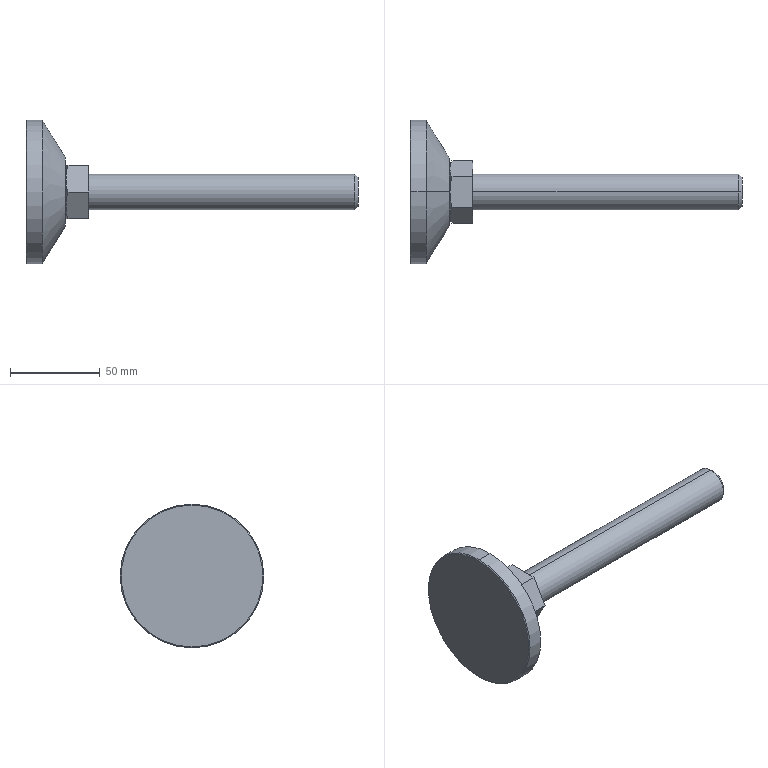Part | SolidWorks | features BaseBody 1 | 1 solid | 22 faces | box 185 x 80 x 80 mm | volume 139335 mm3 | plane 10 | cone 6 | cylinder 4 | spline 2 | commonest cylinder face diameters 20 x2 80 x2
STEP:
#1=CARTESIAN_POINT('',(23.401,-8.66,15.));
#2=VERTEX_POINT('',#1);
#3=CARTESIAN_POINT('',(22.274,0.,15.));
#4=VERTEX_POINT('',#3);
#5=CARTESIAN_POINT('',(23.401,-8.66,15.));
#6=CARTESIAN_POINT('',(23.148,-7.966,15.));
#7=CARTESIAN_POINT('',(22.959,-7.26,15.));
#8=CARTESIAN_POINT('',(22.664,-5.832,15.));
#9=CARTESIAN_POINT('',(22.559,-5.11,15.));
#10=CARTESIAN_POINT('',(22.403,-3.657,15.));
#11=CARTESIAN_POINT('',(22.353,-2.924,15.));
#12=CARTESIAN_POINT('',(22.288,-1.461,15.));
#13=CARTESIAN_POINT('',(22.274,-0.73,15.));
#14=CARTESIAN_POINT('',(22.274,0.,15.));
#15=B_SPLINE_CURVE_WITH_KNOTS('',3,(#5,#6,#7,#8,#9,#10,#11,#12,#13,#14),.UNSPECIFIED.,.F.,.F.,(4,2,2,2,4),(0.,0.002186,0.004373,0.006559,0.008745),.UNSPECIFIED.);
#16=EDGE_CURVE('',#2,#4,#15,.T.);
#17=ORIENTED_EDGE('',*,*,#16,.T.);
#18=CARTESIAN_POINT('',(22.,0.,13.021));
#19=VERTEX_POINT('',#18);
#20=CARTESIAN_POINT('',(29.3,0.,13.021));
#21=DIRECTION('',(0.,-1.,0.));
#22=DIRECTION('',(0.,0.,1.));
#23=AXIS2_PLACEMENT_3D('',#20,#21,#22);
#24=CIRCLE('',#23,7.3);
#25=EDGE_CURVE('',#4,#19,#24,.T.);
#26=ORIENTED_EDGE('',*,*,#25,.T.);
#27=CARTESIAN_POINT('',(22.,0.,-13.021));
#28=VERTEX_POINT('',#27);
#29=CARTESIAN_POINT('',(22.,0.,13.021));
#30=CARTESIAN_POINT('',(22.,-26.041,13.021));
#31=CARTESIAN_POINT('',(22.,-26.041,-13.021));
#32=CARTESIAN_POINT('',(22.,0.,-13.021));
#33=(BOUNDED_CURVE()B_SPLINE_CURVE(3,(#29,#30,#31,#32),.UNSPECIFIED.,.F.,.F.)B_SPLINE_CURVE_WITH_KNOTS((4,4),(0.5,1.),.UNSPECIFIED.)CURVE()GEOMETRIC_REPRESENTATION_ITEM()RATIONAL_B_SPLINE_CURVE((1.,0.3333,0.3333,1.))REPRESENTATION_ITEM(''));
#34=EDGE_CURVE('',#19,#28,#33,.T.);
#35=ORIENTED_EDGE('',*,*,#34,.T.);
#36=CARTESIAN_POINT('',(22.274,0.,-15.));
#37=VERTEX_POINT('',#36);
#38=CARTESIAN_POINT('',(29.3,0.,-13.021));
#39=DIRECTION('',(0.,1.,0.));
#40=DIRECTION('',(0.,0.,-1.));
#41=AXIS2_PLACEMENT_3D('',#38,#39,#40);
#42=CIRCLE('',#41,7.3);
#43=EDGE_CURVE('',#37,#28,#42,.T.);
#44=ORIENTED_EDGE('',*,*,#43,.F.);
#45=CARTESIAN_POINT('',(23.401,-8.66,-15.));
#46=VERTEX_POINT('',#45);
#47=CARTESIAN_POINT('',(22.274,0.,-15.));
#48=CARTESIAN_POINT('',(22.274,-0.7289,-15.));
#49=CARTESIAN_POINT('',(22.288,-1.457,-15.));
#50=CARTESIAN_POINT('',(22.352,-2.912,-15.));
#51=CARTESIAN_POINT('',(22.402,-3.638,-15.));
#52=CARTESIAN_POINT('',(22.556,-5.089,-15.));
#53=CARTESIAN_POINT('',(22.661,-5.813,-15.));
#54=CARTESIAN_POINT('',(22.958,-7.257,-15.));
#55=CARTESIAN_POINT('',(23.148,-7.967,-15.));
#56=CARTESIAN_POINT('',(23.401,-8.66,-15.));
#57=B_SPLINE_CURVE_WITH_KNOTS('',3,(#47,#48,#49,#50,#51,#52,#53,#54,#55,#56),.UNSPECIFIED.,.F.,.F.,(4,2,2,2,4),(0.008745,0.01093,0.01311,0.01529,0.01748),.UNSPECIFIED.);
#58=EDGE_CURVE('',#37,#46,#57,.T.);
#59=ORIENTED_EDGE('',*,*,#58,.T.);
#60=CARTESIAN_POINT('',(23.401,-17.321,0.));
#61=VERTEX_POINT('',#60);
#62=CARTESIAN_POINT('',(23.401,-8.66,-15.));
#63=CARTESIAN_POINT('',(23.148,-9.007,-14.399));
#64=CARTESIAN_POINT('',(22.959,-9.36,-13.788));
#65=CARTESIAN_POINT('',(22.665,-10.073,-12.552));
#66=CARTESIAN_POINT('',(22.56,-10.434,-11.928));
#67=CARTESIAN_POINT('',(22.404,-11.16,-10.67));
#68=CARTESIAN_POINT('',(22.353,-11.526,-10.036));
#69=CARTESIAN_POINT('',(22.288,-12.257,-8.77));
#70=CARTESIAN_POINT('',(22.274,-12.622,-8.138));
#71=CARTESIAN_POINT('',(22.273,-13.352,-6.874));
#72=CARTESIAN_POINT('',(22.288,-13.716,-6.243));
#73=CARTESIAN_POINT('',(22.352,-14.444,-4.982));
#74=CARTESIAN_POINT('',(22.402,-14.808,-4.353));
#75=CARTESIAN_POINT('',(22.556,-15.533,-3.095));
#76=CARTESIAN_POINT('',(22.661,-15.896,-2.468));
#77=CARTESIAN_POINT('',(22.958,-16.618,-1.216));
#78=CARTESIAN_POINT('',(23.148,-16.974,-0.6006));
#79=CARTESIAN_POINT('',(23.401,-17.321,0.));
#80=B_SPLINE_CURVE_WITH_KNOTS('',3,(#62,#63,#64,#65,#66,#67,#68,#69,#70,#71,#72,#73,#74,#75,#76,#77,#78,#79),.UNSPECIFIED.,.F.,.F.,(4,2,2,2,2,2,2,2,4),(0.,0.002185,0.004369,0.006554,0.008739,0.01092,0.01311,0.01529,0.01748),.UNSPECIFIED.);
#81=EDGE_CURVE('',#46,#61,#80,.T.);
#82=ORIENTED_EDGE('',*,*,#81,.T.);
#83=CARTESIAN_POINT('',(23.401,-17.321,0.));
#84=CARTESIAN_POINT('',(23.148,-16.974,0.6009));
#85=CARTESIAN_POINT('',(22.959,-16.621,1.212));
#86=CARTESIAN_POINT('',(22.665,-15.907,2.448));
#87=CARTESIAN_POINT('',(22.56,-15.547,3.072));
#88=CARTESIAN_POINT('',(22.404,-14.821,4.33));
#89=CARTESIAN_POINT('',(22.353,-14.454,4.964));
#90=CARTESIAN_POINT('',(22.288,-13.723,6.23));
#91=CARTESIAN_POINT('',(22.274,-13.358,6.862));
#92=CARTESIAN_POINT('',(22.273,-12.629,8.126));
#93=CARTESIAN_POINT('',(22.288,-12.265,8.757));
#94=CARTESIAN_POINT('',(22.352,-11.537,10.018));
#95=CARTESIAN_POINT('',(22.402,-11.173,10.647));
#96=CARTESIAN_POINT('',(22.556,-10.447,11.905));
#97=CARTESIAN_POINT('',(22.661,-10.085,12.532));
#98=CARTESIAN_POINT('',(22.958,-9.363,13.784));
#99=CARTESIAN_POINT('',(23.148,-9.007,14.399));
#100=CARTESIAN_POINT('',(23.401,-8.66,15.));
#101=B_SPLINE_CURVE_WITH_KNOTS('',3,(#83,#84,#85,#86,#87,#88,#89,#90,#91,#92,#93,#94,#95,#96,#97,#98,#99,#100),.UNSPECIFIED.,.F.,.F.,(4,2,2,2,2,2,2,2,4),(0.,0.002185,0.004369,0.006554,0.008739,0.01092,0.01311,0.01529,0.01748),.UNSPECIFIED.);
#102=EDGE_CURVE('',#61,#2,#101,.T.);
#103=ORIENTED_EDGE('',*,*,#102,.T.);
#104=EDGE_LOOP('',(#17,#26,#35,#44,#59,#82,#103));
#105=FACE_OUTER_BOUND('',#104,.T.);
#106=CARTESIAN_POINT('',(23.417,0.,17.343));
#107=CARTESIAN_POINT('',(23.417,-34.686,17.343));
#108=CARTESIAN_POINT('',(23.417,-34.686,-17.343));
#109=CARTESIAN_POINT('',(23.417,0.,-17.343));
#110=CARTESIAN_POINT('',(22.489,0.,16.079));
#111=CARTESIAN_POINT('',(22.489,-32.158,16.079));
#112=CARTESIAN_POINT('',(22.489,-32.158,-16.079));
#113=CARTESIAN_POINT('',(22.489,0.,-16.079));
#114=CARTESIAN_POINT('',(22.,0.,14.589));
#115=CARTESIAN_POINT('',(22.,-29.178,14.589));
#116=CARTESIAN_POINT('',(22.,-29.178,-14.589));
#117=CARTESIAN_POINT('',(22.,0.,-14.589));
#118=CARTESIAN_POINT('',(22.,0.,13.021));
#119=CARTESIAN_POINT('',(22.,-26.041,13.021));
#120=CARTESIAN_POINT('',(22.,-26.041,-13.021));
#121=CARTESIAN_POINT('',(22.,0.,-13.021));
#122=(BOUNDED_SURFACE()B_SPLINE_SURFACE(3,3,((#106,#107,#108,#109),(#110,#111,#112,#113),(#114,#115,#116,#117),(#118,#119,#120,#121)),.UNSPECIFIED.,.F.,.F.,.F.)B_SPLINE_SURFACE_WITH_KNOTS((4,4),(4,4),(0.,1.),(0.,1.),.UNSPECIFIED.)GEOMETRIC_REPRESENTATION_ITEM()RATIONAL_B_SPLINE_SURFACE(((1.,0.3333,0.3333,1.),(0.9668,0.3223,0.3223,0.9668),(0.9668,0.3223,0.3223,0.9668),(1.,0.3333,0.3333,1.)))REPRESENTATION_ITEM('')SURFACE());
#123=ADVANCED_FACE('',(#105),#122,.T.);
#124=CARTESIAN_POINT('',(35.,0.,-10.));
#125=VERTEX_POINT('',#124);
#126=CARTESIAN_POINT('',(35.,0.,10.));
#127=VERTEX_POINT('',#126);
#128=CARTESIAN_POINT('',(35.,0.,0.));
#129=DIRECTION('',(1.,0.,0.));
#130=DIRECTION('',(0.,0.,-1.));
#131=AXIS2_PLACEMENT_3D('',#128,#129,#130);
#132=CIRCLE('',#131,10.);
#133=EDGE_CURVE('',#125,#127,#132,.T.);
#134=ORIENTED_EDGE('',*,*,#133,.T.);
#135=CARTESIAN_POINT('',(183.,0.,10.));
#136=VERTEX_POINT('',#135);
#137=CARTESIAN_POINT('',(185.,0.,10.));
#138=DIRECTION('',(1.,0.,0.));
#139=VECTOR('',#138,1000.);
#140=LINE('',#137,#139);
#141=EDGE_CURVE('',#127,#136,#140,.T.);
#142=ORIENTED_EDGE('',*,*,#141,.T.);
#143=CARTESIAN_POINT('',(183.,0.,-10.));
#144=VERTEX_POINT('',#143);
#145=CARTESIAN_POINT('',(183.,0.,0.));
#146=DIRECTION('',(-1.,0.,0.));
#147=DIRECTION('',(0.,0.,-1.));
#148=AXIS2_PLACEMENT_3D('',#145,#146,#147);
#149=CIRCLE('',#148,10.);
#150=EDGE_CURVE('',#136,#144,#149,.T.);
#151=ORIENTED_EDGE('',*,*,#150,.T.);
#152=CARTESIAN_POINT('',(185.,0.,-10.));
#153=DIRECTION('',(1.,0.,0.));
#154=VECTOR('',#153,1000.);
#155=LINE('',#152,#154);
#156=EDGE_CURVE('',#125,#144,#155,.T.);
#157=ORIENTED_EDGE('',*,*,#156,.F.);
#158=EDGE_LOOP('',(#134,#142,#151,#157));
#159=FACE_OUTER_BOUND('',#158,.T.);
#160=CARTESIAN_POINT('',(185.,0.,0.));
#161=DIRECTION('',(1.,0.,0.));
#162=DIRECTION('',(0.,0.,-1.));
#163=AXIS2_PLACEMENT_3D('',#160,#161,#162);
#164=CYLINDRICAL_SURFACE('',#163,10.);
#165=ADVANCED_FACE('',(#159),#164,.T.);
#166=CARTESIAN_POINT('',(185.,0.,8.));
#167=VERTEX_POINT('',#166);
#168=CARTESIAN_POINT('',(185.,0.,-8.));
#169=VERTEX_POINT('',#168);
#170=CARTESIAN_POINT('',(185.,0.,0.));
#171=DIRECTION('',(-1.,0.,0.));
#172=DIRECTION('',(0.,0.,1.));
#173=AXIS2_PLACEMENT_3D('',#170,#171,#172);
#174=CIRCLE('',#173,8.);
#175=EDGE_CURVE('',#167,#169,#174,.T.);
#176=ORIENTED_EDGE('',*,*,#175,.T.);
#177=CARTESIAN_POINT('',(183.,0.,-10.));
#178=DIRECTION('',(-0.7071,0.,-0.7071));
#179=VECTOR('',#178,1000.);
#180=LINE('',#177,#179);
#181=EDGE_CURVE('',#169,#144,#180,.T.);
#182=ORIENTED_EDGE('',*,*,#181,.T.);
#183=ORIENTED_EDGE('',*,*,#150,.F.);
#184=CARTESIAN_POINT('',(183.,0.,10.));
#185=DIRECTION('',(-0.7071,0.,0.7071));
#186=VECTOR('',#185,1000.);
#187=LINE('',#184,#186);
#188=EDGE_CURVE('',#167,#136,#187,.T.);
#189=ORIENTED_EDGE('',*,*,#188,.F.);
#190=EDGE_LOOP('',(#176,#182,#183,#189));
#191=FACE_OUTER_BOUND('',#190,.T.);
#192=CARTESIAN_POINT('',(183.,0.,0.));
#193=DIRECTION('',(-1.,0.,0.));
#194=DIRECTION('',(0.,0.,1.));
#195=AXIS2_PLACEMENT_3D('',#192,#193,#194);
#196=CONICAL_SURFACE('',#195,10.,0.7854);
#197=ADVANCED_FACE('',(#191),#196,.T.);
#198=CARTESIAN_POINT('',(22.,0.,19.));
#199=VERTEX_POINT('',#198);
#200=CARTESIAN_POINT('',(22.,0.,-19.));
#201=VERTEX_POINT('',#200);
#202=CARTESIAN_POINT('',(22.,0.,0.));
#203=DIRECTION('',(-1.,0.,0.));
#204=DIRECTION('',(0.,0.,1.));
#205=AXIS2_PLACEMENT_3D('',#202,#203,#204);
#206=CIRCLE('',#205,19.);
#207=EDGE_CURVE('',#199,#201,#206,.T.);
#208=ORIENTED_EDGE('',*,*,#207,.T.);
#209=CARTESIAN_POINT('',(9.,0.,-40.));
#210=VERTEX_POINT('',#209);
#211=CARTESIAN_POINT('',(9.,0.,-40.));
#212=DIRECTION('',(-0.5264,0.,-0.8503));
#213=VECTOR('',#212,1000.);
#214=LINE('',#211,#213);
#215=EDGE_CURVE('',#201,#210,#214,.T.);
#216=ORIENTED_EDGE('',*,*,#215,.T.);
#217=CARTESIAN_POINT('',(9.,0.,40.));
#218=VERTEX_POINT('',#217);
#219=CARTESIAN_POINT('',(9.,0.,0.));
#220=DIRECTION('',(1.,0.,0.));
#221=DIRECTION('',(0.,0.,1.));
#222=AXIS2_PLACEMENT_3D('',#219,#220,#221);
#223=CIRCLE('',#222,40.);
#224=EDGE_CURVE('',#210,#218,#223,.T.);
#225=ORIENTED_EDGE('',*,*,#224,.T.);
#226=CARTESIAN_POINT('',(9.,0.,40.));
#227=DIRECTION('',(-0.5264,0.,0.8503));
#228=VECTOR('',#227,1000.);
#229=LINE('',#226,#228);
#230=EDGE_CURVE('',#199,#218,#229,.T.);
#231=ORIENTED_EDGE('',*,*,#230,.F.);
#232=EDGE_LOOP('',(#208,#216,#225,#231));
#233=FACE_OUTER_BOUND('',#232,.T.);
#234=CARTESIAN_POINT('',(9.,0.,0.));
#235=DIRECTION('',(-1.,0.,0.));
#236=DIRECTION('',(0.,0.,1.));
#237=AXIS2_PLACEMENT_3D('',#234,#235,#236);
#238=CONICAL_SURFACE('',#237,40.,1.016);
#239=ADVANCED_FACE('',(#233),#238,.T.);
#240=CARTESIAN_POINT('',(0.5,0.,-40.));
#241=VERTEX_POINT('',#240);
#242=CARTESIAN_POINT('',(0.5,0.,40.));
#243=VERTEX_POINT('',#242);
#244=CARTESIAN_POINT('',(0.5,0.,0.));
#245=DIRECTION('',(1.,0.,0.));
#246=DIRECTION('',(0.,0.,-1.));
#247=AXIS2_PLACEMENT_3D('',#244,#245,#246);
#248=CIRCLE('',#247,40.);
#249=EDGE_CURVE('',#241,#243,#248,.T.);
#250=ORIENTED_EDGE('',*,*,#249,.T.);
#251=CARTESIAN_POINT('',(185.,0.,40.));
#252=DIRECTION('',(1.,0.,0.));
#253=VECTOR('',#252,1000.);
#254=LINE('',#251,#253);
#255=EDGE_CURVE('',#243,#218,#254,.T.);
#256=ORIENTED_EDGE('',*,*,#255,.T.);
#257=ORIENTED_EDGE('',*,*,#224,.F.);
#258=CARTESIAN_POINT('',(185.,0.,-40.));
#259=DIRECTION('',(1.,0.,0.));
#260=VECTOR('',#259,1000.);
#261=LINE('',#258,#260);
#262=EDGE_CURVE('',#241,#210,#261,.T.);
#263=ORIENTED_EDGE('',*,*,#262,.F.);
#264=EDGE_LOOP('',(#250,#256,#257,#263));
#265=FACE_OUTER_BOUND('',#264,.T.);
#266=CARTESIAN_POINT('',(185.,0.,0.));
#267=DIRECTION('',(1.,0.,0.));
#268=DIRECTION('',(0.,0.,-1.));
#269=AXIS2_PLACEMENT_3D('',#266,#267,#268);
#270=CYLINDRICAL_SURFACE('',#269,40.);
#271=ADVANCED_FACE('',(#265),#270,.T.);
#272=CARTESIAN_POINT('',(0.,0.,-39.5));
#273=VERTEX_POINT('',#272);
#274=CARTESIAN_POINT('',(0.,0.,39.5));
#275=VERTEX_POINT('',#274);
#276=CARTESIAN_POINT('',(0.,0.,0.));
#277=DIRECTION('',(1.,0.,0.));
#278=DIRECTION('',(0.,0.,-1.));
#279=AXIS2_PLACEMENT_3D('',#276,#277,#278);
#280=CIRCLE('',#279,39.5);
#281=EDGE_CURVE('',#273,#275,#280,.T.);
#282=ORIENTED_EDGE('',*,*,#281,.T.);
#283=CARTESIAN_POINT('',(0.5,0.,40.));
#284=DIRECTION('',(0.7071,0.,0.7071));
#285=VECTOR('',#284,1000.);
#286=LINE('',#283,#285);
#287=EDGE_CURVE('',#275,#243,#286,.T.);
#288=ORIENTED_EDGE('',*,*,#287,.T.);
#289=ORIENTED_EDGE('',*,*,#249,.F.);
#290=CARTESIAN_POINT('',(0.5,0.,-40.));
#291=DIRECTION('',(0.7071,0.,-0.7071));
#292=VECTOR('',#291,1000.);
#293=LINE('',#290,#292);
#294=EDGE_CURVE('',#273,#241,#293,.T.);
#295=ORIENTED_EDGE('',*,*,#294,.F.);
#296=EDGE_LOOP('',(#282,#288,#289,#295));
#297=FACE_OUTER_BOUND('',#296,.T.);
#298=CARTESIAN_POINT('',(0.5,0.,0.));
#299=DIRECTION('',(1.,0.,0.));
#300=DIRECTION('',(0.,0.,-1.));
#301=AXIS2_PLACEMENT_3D('',#298,#299,#300);
#302=CONICAL_SURFACE('',#301,40.,0.7854);
#303=ADVANCED_FACE('',(#297),#302,.T.);
#304=ORIENTED_EDGE('',*,*,#141,.F.);
#305=CARTESIAN_POINT('',(35.,0.,0.));
#306=DIRECTION('',(1.,0.,0.));
#307=DIRECTION('',(0.,0.,-1.));
#308=AXIS2_PLACEMENT_3D('',#305,#306,#307);
#309=CIRCLE('',#308,10.);
#310=EDGE_CURVE('',#127,#125,#309,.T.);
#311=ORIENTED_EDGE('',*,*,#310,.T.);
#312=ORIENTED_EDGE('',*,*,#156,.T.);
#313=CARTESIAN_POINT('',(183.,0.,0.));
#314=DIRECTION('',(-1.,0.,0.));
#315=DIRECTION('',(0.,0.,-1.));
#316=AXIS2_PLACEMENT_3D('',#313,#314,#315);
#317=CIRCLE('',#316,10.);
#318=EDGE_CURVE('',#144,#136,#317,.T.);
#319=ORIENTED_EDGE('',*,*,#318,.T.);
#320=EDGE_LOOP('',(#304,#311,#312,#319));
#321=FACE_OUTER_BOUND('',#320,.T.);
#322=CARTESIAN_POINT('',(185.,0.,0.));
#323=DIRECTION('',(1.,0.,0.));
#324=DIRECTION('',(0.,0.,-1.));
#325=AXIS2_PLACEMENT_3D('',#322,#323,#324);
#326=CYLINDRICAL_SURFACE('',#325,10.);
#327=ADVANCED_FACE('',(#321),#326,.T.);
#328=CARTESIAN_POINT('',(35.,-8.66,15.));
#329=VERTEX_POINT('',#328);
#330=CARTESIAN_POINT('',(35.,8.66,15.));
#331=VERTEX_POINT('',#330);
#332=CARTESIAN_POINT('',(35.,17.321,15.));
#333=DIRECTION('',(0.,1.,0.));
#334=VECTOR('',#333,1000.);
#335=LINE('',#332,#334);
#336=EDGE_CURVE('',#329,#331,#335,.T.);
#337=ORIENTED_EDGE('',*,*,#336,.F.);
#338=CARTESIAN_POINT('',(35.,-17.321,0.));
#339=VERTEX_POINT('',#338);
#340=CARTESIAN_POINT('',(35.,-17.321,0.));
#341=DIRECTION('',(0.,0.5,0.866));
#342=VECTOR('',#341,1000.);
#343=LINE('',#340,#342);
#344=EDGE_CURVE('',#339,#329,#343,.T.);
#345=ORIENTED_EDGE('',*,*,#344,.F.);
#346=CARTESIAN_POINT('',(35.,-8.66,-15.));
#347=VERTEX_POINT('',#346);
#348=CARTESIAN_POINT('',(35.,-8.66,-15.));
#349=DIRECTION('',(0.,-0.5,0.866));
#350=VECTOR('',#349,1000.);
#351=LINE('',#348,#350);
#352=EDGE_CURVE('',#347,#339,#351,.T.);
#353=ORIENTED_EDGE('',*,*,#352,.F.);
#354=CARTESIAN_POINT('',(35.,8.66,-15.));
#355=VERTEX_POINT('',#354);
#356=CARTESIAN_POINT('',(35.,17.321,-15.));
#357=DIRECTION('',(0.,-1.,0.));
#358=VECTOR('',#357,1000.);
#359=LINE('',#356,#358);
#360=EDGE_CURVE('',#355,#347,#359,.T.);
#361=ORIENTED_EDGE('',*,*,#360,.F.);
#362=CARTESIAN_POINT('',(35.,17.321,0.));
#363=VERTEX_POINT('',#362);
#364=CARTESIAN_POINT('',(35.,17.321,0.));
#365=DIRECTION('',(0.,-0.5,-0.866));
#366=VECTOR('',#365,1000.);
#367=LINE('',#364,#366);
#368=EDGE_CURVE('',#363,#355,#367,.T.);
#369=ORIENTED_EDGE('',*,*,#368,.F.);
#370=CARTESIAN_POINT('',(35.,8.66,15.));
#371=DIRECTION('',(0.,0.5,-0.866));
#372=VECTOR('',#371,1000.);
#373=LINE('',#370,#372);
#374=EDGE_CURVE('',#331,#363,#373,.T.);
#375=ORIENTED_EDGE('',*,*,#374,.F.);
#376=EDGE_LOOP('',(#337,#345,#353,#361,#369,#375));
#377=FACE_OUTER_BOUND('',#376,.T.);
#378=ORIENTED_EDGE('',*,*,#133,.F.);
#379=ORIENTED_EDGE('',*,*,#310,.F.);
#380=EDGE_LOOP('',(#378,#379));
#381=FACE_BOUND('',#380,.T.);
#382=CARTESIAN_POINT('',(35.,17.321,0.));
#383=DIRECTION('',(-1.,0.,0.));
#384=DIRECTION('',(0.,0.,1.));
#385=AXIS2_PLACEMENT_3D('',#382,#383,#384);
#386=PLANE('',#385);
#387=ADVANCED_FACE('',(#377,#381),#386,.F.);
#388=ORIENTED_EDGE('',*,*,#181,.F.);
#389=CARTESIAN_POINT('',(185.,0.,0.));
#390=DIRECTION('',(-1.,0.,0.));
#391=DIRECTION('',(0.,0.,1.));
#392=AXIS2_PLACEMENT_3D('',#389,#390,#391);
#393=CIRCLE('',#392,8.);
#394=EDGE_CURVE('',#169,#167,#393,.T.);
#395=ORIENTED_EDGE('',*,*,#394,.T.);
#396=ORIENTED_EDGE('',*,*,#188,.T.);
#397=ORIENTED_EDGE('',*,*,#318,.F.);
#398=EDGE_LOOP('',(#388,#395,#396,#397));
#399=FACE_OUTER_BOUND('',#398,.T.);
#400=CARTESIAN_POINT('',(183.,0.,0.));
#401=DIRECTION('',(-1.,0.,0.));
#402=DIRECTION('',(0.,0.,1.));
#403=AXIS2_PLACEMENT_3D('',#400,#401,#402);
#404=CONICAL_SURFACE('',#403,10.,0.7854);
#405=ADVANCED_FACE('',(#399),#404,.T.);
#406=CARTESIAN_POINT('',(23.401,8.66,15.));
#407=VERTEX_POINT('',#406);
#408=CARTESIAN_POINT('',(35.,8.66,15.));
#409=DIRECTION('',(-1.,0.,0.));
#410=VECTOR('',#409,1000.);
#411=LINE('',#408,#410);
#412=EDGE_CURVE('',#331,#407,#411,.T.);
#413=ORIENTED_EDGE('',*,*,#412,.F.);
#414=ORIENTED_EDGE('',*,*,#374,.T.);
#415=CARTESIAN_POINT('',(23.401,17.321,0.));
#416=VERTEX_POINT('',#415);
#417=CARTESIAN_POINT('',(35.,17.321,0.));
#418=DIRECTION('',(1.,0.,0.));
#419=VECTOR('',#418,1000.);
#420=LINE('',#417,#419);
#421=EDGE_CURVE('',#416,#363,#420,.T.);
#422=ORIENTED_EDGE('',*,*,#421,.F.);
#423=CARTESIAN_POINT('',(23.401,8.66,15.));
#424=CARTESIAN_POINT('',(23.148,9.007,14.399));
#425=CARTESIAN_POINT('',(22.959,9.36,13.788));
#426=CARTESIAN_POINT('',(22.665,10.073,12.552));
#427=CARTESIAN_POINT('',(22.56,10.434,11.928));
#428=CARTESIAN_POINT('',(22.404,11.16,10.67));
#429=CARTESIAN_POINT('',(22.353,11.526,10.036));
#430=CARTESIAN_POINT('',(22.288,12.257,8.77));
#431=CARTESIAN_POINT('',(22.274,12.622,8.138));
#432=CARTESIAN_POINT('',(22.273,13.352,6.874));
#433=CARTESIAN_POINT('',(22.288,13.716,6.243));
#434=CARTESIAN_POINT('',(22.352,14.444,4.982));
#435=CARTESIAN_POINT('',(22.402,14.808,4.353));
#436=CARTESIAN_POINT('',(22.556,15.533,3.095));
#437=CARTESIAN_POINT('',(22.661,15.896,2.468));
#438=CARTESIAN_POINT('',(22.958,16.618,1.216));
#439=CARTESIAN_POINT('',(23.148,16.974,0.6006));
#440=CARTESIAN_POINT('',(23.401,17.321,0.));
#441=B_SPLINE_CURVE_WITH_KNOTS('',3,(#423,#424,#425,#426,#427,#428,#429,#430,#431,#432,#433,#434,#435,#436,#437,#438,#439,#440),.UNSPECIFIED.,.F.,.F.,(4,2,2,2,2,2,2,2,4),(0.,0.002185,0.004369,0.006554,0.008739,0.01092,0.01311,0.01529,0.01748),.UNSPECIFIED.);
#442=EDGE_CURVE('',#407,#416,#441,.T.);
#443=ORIENTED_EDGE('',*,*,#442,.F.);
#444=EDGE_LOOP('',(#413,#414,#422,#443));
#445=FACE_OUTER_BOUND('',#444,.T.);
#446=CARTESIAN_POINT('',(35.,17.321,0.));
#447=DIRECTION('',(0.,-0.866,-0.5));
#448=DIRECTION('',(0.,0.5,-0.866));
#449=AXIS2_PLACEMENT_3D('',#446,#447,#448);
#450=PLANE('',#449);
#451=ADVANCED_FACE('',(#445),#450,.F.);
#452=CARTESIAN_POINT('',(35.,-8.66,15.));
#453=DIRECTION('',(-1.,0.,0.));
#454=VECTOR('',#453,1000.);
#455=LINE('',#452,#454);
#456=EDGE_CURVE('',#329,#2,#455,.T.);
#457=ORIENTED_EDGE('',*,*,#456,.F.);
#458=ORIENTED_EDGE('',*,*,#336,.T.);
#459=ORIENTED_EDGE('',*,*,#412,.T.);
#460=CARTESIAN_POINT('',(22.274,0.,15.));
#461=CARTESIAN_POINT('',(22.274,0.7289,15.));
#462=CARTESIAN_POINT('',(22.288,1.457,15.));
#463=CARTESIAN_POINT('',(22.352,2.912,15.));
#464=CARTESIAN_POINT('',(22.402,3.638,15.));
#465=CARTESIAN_POINT('',(22.556,5.089,15.));
#466=CARTESIAN_POINT('',(22.661,5.813,15.));
#467=CARTESIAN_POINT('',(22.958,7.257,15.));
#468=CARTESIAN_POINT('',(23.148,7.967,15.));
#469=CARTESIAN_POINT('',(23.401,8.66,15.));
#470=B_SPLINE_CURVE_WITH_KNOTS('',3,(#460,#461,#462,#463,#464,#465,#466,#467,#468,#469),.UNSPECIFIED.,.F.,.F.,(4,2,2,2,4),(0.008745,0.01093,0.01311,0.01529,0.01748),.UNSPECIFIED.);
#471=EDGE_CURVE('',#4,#407,#470,.T.);
#472=ORIENTED_EDGE('',*,*,#471,.F.);
#473=ORIENTED_EDGE('',*,*,#16,.F.);
#474=EDGE_LOOP('',(#457,#458,#459,#472,#473));
#475=FACE_OUTER_BOUND('',#474,.T.);
#476=CARTESIAN_POINT('',(35.,8.66,15.));
#477=DIRECTION('',(0.,0.,-1.));
#478=DIRECTION('',(-1.,0.,0.));
#479=AXIS2_PLACEMENT_3D('',#476,#477,#478);
#480=PLANE('',#479);
#481=ADVANCED_FACE('',(#475),#480,.F.);
#482=CARTESIAN_POINT('',(35.,-17.321,0.));
#483=DIRECTION('',(-1.,0.,0.));
#484=VECTOR('',#483,1000.);
#485=LINE('',#482,#484);
#486=EDGE_CURVE('',#339,#61,#485,.T.);
#487=ORIENTED_EDGE('',*,*,#486,.F.);
#488=ORIENTED_EDGE('',*,*,#344,.T.);
#489=ORIENTED_EDGE('',*,*,#456,.T.);
#490=ORIENTED_EDGE('',*,*,#102,.F.);
#491=EDGE_LOOP('',(#487,#488,#489,#490));
#492=FACE_OUTER_BOUND('',#491,.T.);
#493=CARTESIAN_POINT('',(35.,-8.66,15.));
#494=DIRECTION('',(0.,0.866,-0.5));
#495=DIRECTION('',(0.,0.5,0.866));
#496=AXIS2_PLACEMENT_3D('',#493,#494,#495);
#497=PLANE('',#496);
#498=ADVANCED_FACE('',(#492),#497,.F.);
#499=CARTESIAN_POINT('',(35.,-8.66,-15.));
#500=DIRECTION('',(-1.,0.,0.));
#501=VECTOR('',#500,1000.);
#502=LINE('',#499,#501);
#503=EDGE_CURVE('',#347,#46,#502,.T.);
#504=ORIENTED_EDGE('',*,*,#503,.F.);
#505=ORIENTED_EDGE('',*,*,#352,.T.);
#506=ORIENTED_EDGE('',*,*,#486,.T.);
#507=ORIENTED_EDGE('',*,*,#81,.F.);
#508=EDGE_LOOP('',(#504,#505,#506,#507));
#509=FACE_OUTER_BOUND('',#508,.T.);
#510=CARTESIAN_POINT('',(35.,-17.321,0.));
#511=DIRECTION('',(0.,0.866,0.5));
#512=DIRECTION('',(0.,-0.5,0.866));
#513=AXIS2_PLACEMENT_3D('',#510,#511,#512);
#514=PLANE('',#513);
#515=ADVANCED_FACE('',(#509),#514,.F.);
#516=CARTESIAN_POINT('',(23.401,8.66,-15.));
#517=VERTEX_POINT('',#516);
#518=CARTESIAN_POINT('',(35.,8.66,-15.));
#519=DIRECTION('',(-1.,0.,0.));
#520=VECTOR('',#519,1000.);
#521=LINE('',#518,#520);
#522=EDGE_CURVE('',#355,#517,#521,.T.);
#523=ORIENTED_EDGE('',*,*,#522,.F.);
#524=ORIENTED_EDGE('',*,*,#360,.T.);
#525=ORIENTED_EDGE('',*,*,#503,.T.);
#526=ORIENTED_EDGE('',*,*,#58,.F.);
#527=CARTESIAN_POINT('',(23.401,8.66,-15.));
#528=CARTESIAN_POINT('',(23.148,7.966,-15.));
#529=CARTESIAN_POINT('',(22.959,7.26,-15.));
#530=CARTESIAN_POINT('',(22.664,5.832,-15.));
#531=CARTESIAN_POINT('',(22.559,5.11,-15.));
#532=CARTESIAN_POINT('',(22.403,3.657,-15.));
#533=CARTESIAN_POINT('',(22.353,2.924,-15.));
#534=CARTESIAN_POINT('',(22.288,1.461,-15.));
#535=CARTESIAN_POINT('',(22.274,0.73,-15.));
#536=CARTESIAN_POINT('',(22.274,0.,-15.));
#537=B_SPLINE_CURVE_WITH_KNOTS('',3,(#527,#528,#529,#530,#531,#532,#533,#534,#535,#536),.UNSPECIFIED.,.F.,.F.,(4,2,2,2,4),(0.,0.002186,0.004373,0.006559,0.008745),.UNSPECIFIED.);
#538=EDGE_CURVE('',#517,#37,#537,.T.);
#539=ORIENTED_EDGE('',*,*,#538,.F.);
#540=EDGE_LOOP('',(#523,#524,#525,#526,#539));
#541=FACE_OUTER_BOUND('',#540,.T.);
#542=CARTESIAN_POINT('',(35.,-8.66,-15.));
#543=DIRECTION('',(0.,0.,1.));
#544=DIRECTION('',(1.,0.,0.));
#545=AXIS2_PLACEMENT_3D('',#542,#543,#544);
#546=PLANE('',#545);
#547=ADVANCED_FACE('',(#541),#546,.F.);
#548=ORIENTED_EDGE('',*,*,#421,.T.);
#549=ORIENTED_EDGE('',*,*,#368,.T.);
#550=ORIENTED_EDGE('',*,*,#522,.T.);
#551=CARTESIAN_POINT('',(23.401,17.321,0.));
#552=CARTESIAN_POINT('',(23.148,16.974,-0.6009));
#553=CARTESIAN_POINT('',(22.959,16.621,-1.212));
#554=CARTESIAN_POINT('',(22.665,15.907,-2.448));
#555=CARTESIAN_POINT('',(22.56,15.547,-3.072));
#556=CARTESIAN_POINT('',(22.404,14.821,-4.33));
#557=CARTESIAN_POINT('',(22.353,14.454,-4.964));
#558=CARTESIAN_POINT('',(22.288,13.723,-6.23));
#559=CARTESIAN_POINT('',(22.274,13.358,-6.862));
#560=CARTESIAN_POINT('',(22.273,12.629,-8.126));
#561=CARTESIAN_POINT('',(22.288,12.265,-8.757));
#562=CARTESIAN_POINT('',(22.352,11.537,-10.018));
#563=CARTESIAN_POINT('',(22.402,11.173,-10.647));
#564=CARTESIAN_POINT('',(22.556,10.447,-11.905));
#565=CARTESIAN_POINT('',(22.661,10.085,-12.532));
#566=CARTESIAN_POINT('',(22.958,9.363,-13.784));
#567=CARTESIAN_POINT('',(23.148,9.007,-14.399));
#568=CARTESIAN_POINT('',(23.401,8.66,-15.));
#569=B_SPLINE_CURVE_WITH_KNOTS('',3,(#551,#552,#553,#554,#555,#556,#557,#558,#559,#560,#561,#562,#563,#564,#565,#566,#567,#568),.UNSPECIFIED.,.F.,.F.,(4,2,2,2,2,2,2,2,4),(0.,0.002185,0.004369,0.006554,0.008739,0.01092,0.01311,0.01529,0.01748),.UNSPECIFIED.);
#570=EDGE_CURVE('',#416,#517,#569,.T.);
#571=ORIENTED_EDGE('',*,*,#570,.F.);
#572=EDGE_LOOP('',(#548,#549,#550,#571));
#573=FACE_OUTER_BOUND('',#572,.T.);
#574=CARTESIAN_POINT('',(35.,8.66,-15.));
#575=DIRECTION('',(0.,-0.866,0.5));
#576=DIRECTION('',(0.,-0.5,-0.866));
#577=AXIS2_PLACEMENT_3D('',#574,#575,#576);
#578=PLANE('',#577);
#579=ADVANCED_FACE('',(#573),#578,.F.);
#580=ORIENTED_EDGE('',*,*,#175,.F.);
#581=ORIENTED_EDGE('',*,*,#394,.F.);
#582=EDGE_LOOP('',(#580,#581));
#583=FACE_OUTER_BOUND('',#582,.T.);
#584=CARTESIAN_POINT('',(185.,8.,0.));
#585=DIRECTION('',(-1.,0.,0.));
#586=DIRECTION('',(0.,0.,1.));
#587=AXIS2_PLACEMENT_3D('',#584,#585,#586);
#588=PLANE('',#587);
#589=ADVANCED_FACE('',(#583),#588,.F.);
#590=ORIENTED_EDGE('',*,*,#25,.F.);
#591=ORIENTED_EDGE('',*,*,#471,.T.);
#592=ORIENTED_EDGE('',*,*,#442,.T.);
#593=ORIENTED_EDGE('',*,*,#570,.T.);
#594=ORIENTED_EDGE('',*,*,#538,.T.);
#595=ORIENTED_EDGE('',*,*,#43,.T.);
#596=CARTESIAN_POINT('',(22.,0.,-13.021));
#597=CARTESIAN_POINT('',(22.,26.041,-13.021));
#598=CARTESIAN_POINT('',(22.,26.041,13.021));
#599=CARTESIAN_POINT('',(22.,0.,13.021));
#600=(BOUNDED_CURVE()B_SPLINE_CURVE(3,(#596,#597,#598,#599),.UNSPECIFIED.,.F.,.T.)B_SPLINE_CURVE_WITH_KNOTS((4,4),(0.,0.5),.UNSPECIFIED.)CURVE()GEOMETRIC_REPRESENTATION_ITEM()RATIONAL_B_SPLINE_CURVE((1.,0.3333,0.3333,1.))REPRESENTATION_ITEM(''));
#601=EDGE_CURVE('',#28,#19,#600,.T.);
#602=ORIENTED_EDGE('',*,*,#601,.T.);
#603=EDGE_LOOP('',(#590,#591,#592,#593,#594,#595,#602));
#604=FACE_OUTER_BOUND('',#603,.T.);
#605=CARTESIAN_POINT('',(23.417,0.,-17.343));
#606=CARTESIAN_POINT('',(23.417,34.686,-17.343));
#607=CARTESIAN_POINT('',(23.417,34.686,17.343));
#608=CARTESIAN_POINT('',(23.417,0.,17.343));
#609=CARTESIAN_POINT('',(22.489,0.,-16.079));
#610=CARTESIAN_POINT('',(22.489,32.158,-16.079));
#611=CARTESIAN_POINT('',(22.489,32.158,16.079));
#612=CARTESIAN_POINT('',(22.489,0.,16.079));
#613=CARTESIAN_POINT('',(22.,0.,-14.589));
#614=CARTESIAN_POINT('',(22.,29.178,-14.589));
#615=CARTESIAN_POINT('',(22.,29.178,14.589));
#616=CARTESIAN_POINT('',(22.,0.,14.589));
#617=CARTESIAN_POINT('',(22.,0.,-13.021));
#618=CARTESIAN_POINT('',(22.,26.041,-13.021));
#619=CARTESIAN_POINT('',(22.,26.041,13.021));
#620=CARTESIAN_POINT('',(22.,0.,13.021));
#621=(BOUNDED_SURFACE()B_SPLINE_SURFACE(3,3,((#605,#606,#607,#608),(#609,#610,#611,#612),(#613,#614,#615,#616),(#617,#618,#619,#620)),.UNSPECIFIED.,.F.,.F.,.F.)B_SPLINE_SURFACE_WITH_KNOTS((4,4),(4,4),(0.,1.),(0.,1.),.UNSPECIFIED.)GEOMETRIC_REPRESENTATION_ITEM()RATIONAL_B_SPLINE_SURFACE(((1.,0.3333,0.3333,1.),(0.9668,0.3223,0.3223,0.9668),(0.9668,0.3223,0.3223,0.9668),(1.,0.3333,0.3333,1.)))REPRESENTATION_ITEM('')SURFACE());
#622=ADVANCED_FACE('',(#604),#621,.T.);
#623=ORIENTED_EDGE('',*,*,#207,.F.);
#624=CARTESIAN_POINT('',(22.,0.,0.));
#625=DIRECTION('',(-1.,0.,0.));
#626=DIRECTION('',(0.,0.,1.));
#627=AXIS2_PLACEMENT_3D('',#624,#625,#626);
#628=CIRCLE('',#627,19.);
#629=EDGE_CURVE('',#201,#199,#628,.T.);
#630=ORIENTED_EDGE('',*,*,#629,.F.);
#631=EDGE_LOOP('',(#623,#630));
#632=FACE_OUTER_BOUND('',#631,.T.);
#633=ORIENTED_EDGE('',*,*,#601,.F.);
#634=ORIENTED_EDGE('',*,*,#34,.F.);
#635=EDGE_LOOP('',(#633,#634));
#636=FACE_BOUND('',#635,.T.);
#637=CARTESIAN_POINT('',(22.,19.,0.));
#638=DIRECTION('',(-1.,0.,0.));
#639=DIRECTION('',(0.,0.,1.));
#640=AXIS2_PLACEMENT_3D('',#637,#638,#639);
#641=PLANE('',#640);
#642=ADVANCED_FACE('',(#632,#636),#641,.F.);
#643=ORIENTED_EDGE('',*,*,#215,.F.);
#644=ORIENTED_EDGE('',*,*,#629,.T.);
#645=ORIENTED_EDGE('',*,*,#230,.T.);
#646=CARTESIAN_POINT('',(9.,0.,0.));
#647=DIRECTION('',(1.,0.,0.));
#648=DIRECTION('',(0.,0.,1.));
#649=AXIS2_PLACEMENT_3D('',#646,#647,#648);
#650=CIRCLE('',#649,40.);
#651=EDGE_CURVE('',#218,#210,#650,.T.);
#652=ORIENTED_EDGE('',*,*,#651,.T.);
#653=EDGE_LOOP('',(#643,#644,#645,#652));
#654=FACE_OUTER_BOUND('',#653,.T.);
#655=CARTESIAN_POINT('',(9.,0.,0.));
#656=DIRECTION('',(-1.,0.,0.));
#657=DIRECTION('',(0.,0.,1.));
#658=AXIS2_PLACEMENT_3D('',#655,#656,#657);
#659=CONICAL_SURFACE('',#658,40.,1.016);
#660=ADVANCED_FACE('',(#654),#659,.T.);
#661=ORIENTED_EDGE('',*,*,#255,.F.);
#662=CARTESIAN_POINT('',(0.5,0.,0.));
#663=DIRECTION('',(1.,0.,0.));
#664=DIRECTION('',(0.,0.,-1.));
#665=AXIS2_PLACEMENT_3D('',#662,#663,#664);
#666=CIRCLE('',#665,40.);
#667=EDGE_CURVE('',#243,#241,#666,.T.);
#668=ORIENTED_EDGE('',*,*,#667,.T.);
#669=ORIENTED_EDGE('',*,*,#262,.T.);
#670=ORIENTED_EDGE('',*,*,#651,.F.);
#671=EDGE_LOOP('',(#661,#668,#669,#670));
#672=FACE_OUTER_BOUND('',#671,.T.);
#673=CARTESIAN_POINT('',(185.,0.,0.));
#674=DIRECTION('',(1.,0.,0.));
#675=DIRECTION('',(0.,0.,-1.));
#676=AXIS2_PLACEMENT_3D('',#673,#674,#675);
#677=CYLINDRICAL_SURFACE('',#676,40.);
#678=ADVANCED_FACE('',(#672),#677,.T.);
#679=ORIENTED_EDGE('',*,*,#287,.F.);
#680=CARTESIAN_POINT('',(0.,0.,0.));
#681=DIRECTION('',(1.,0.,0.));
#682=DIRECTION('',(0.,0.,-1.));
#683=AXIS2_PLACEMENT_3D('',#680,#681,#682);
#684=CIRCLE('',#683,39.5);
#685=EDGE_CURVE('',#275,#273,#684,.T.);
#686=ORIENTED_EDGE('',*,*,#685,.T.);
#687=ORIENTED_EDGE('',*,*,#294,.T.);
#688=ORIENTED_EDGE('',*,*,#667,.F.);
#689=EDGE_LOOP('',(#679,#686,#687,#688));
#690=FACE_OUTER_BOUND('',#689,.T.);
#691=CARTESIAN_POINT('',(0.5,0.,0.));
#692=DIRECTION('',(1.,0.,0.));
#693=DIRECTION('',(0.,0.,-1.));
#694=AXIS2_PLACEMENT_3D('',#691,#692,#693);
#695=CONICAL_SURFACE('',#694,40.,0.7854);
#696=ADVANCED_FACE('',(#690),#695,.T.);
#697=ORIENTED_EDGE('',*,*,#281,.F.);
#698=ORIENTED_EDGE('',*,*,#685,.F.);
#699=EDGE_LOOP('',(#697,#698));
#700=FACE_OUTER_BOUND('',#699,.T.);
#701=CARTESIAN_POINT('',(0.,0.,0.));
#702=DIRECTION('',(1.,0.,0.));
#703=DIRECTION('',(0.,0.,-1.));
#704=AXIS2_PLACEMENT_3D('',#701,#702,#703);
#705=PLANE('',#704);
#706=ADVANCED_FACE('',(#700),#705,.F.);
#707=CLOSED_SHELL('',(#123,#165,#197,#239,#271,#303,#327,#387,#405,#451,#481,#498,#515,#547,#579,#589,#622,#642,#660,#678,#696,#706));
#708=MANIFOLD_SOLID_BREP('',#707);
#709=CARTESIAN_POINT('',(0.,0.,0.));
#710=DIRECTION('',(0.,0.,1.));
#711=DIRECTION('',(1.,0.,0.));
#712=AXIS2_PLACEMENT_3D('',#709,#710,#711);
#713=(LENGTH_UNIT()NAMED_UNIT(*)SI_UNIT(.MILLI.,.METRE.));
#714=UNCERTAINTY_MEASURE_WITH_UNIT(LENGTH_MEASURE(0.00001),#713,'','');
#715=(NAMED_UNIT(*)PLANE_ANGLE_UNIT()SI_UNIT($,.RADIAN.));
#716=(NAMED_UNIT(*)SI_UNIT($,.STERADIAN.)SOLID_ANGLE_UNIT());
#717=(GEOMETRIC_REPRESENTATION_CONTEXT(3)GLOBAL_UNCERTAINTY_ASSIGNED_CONTEXT((#714))GLOBAL_UNIT_ASSIGNED_CONTEXT((#713,#715,#716))REPRESENTATION_CONTEXT('',''));
#718=ADVANCED_BREP_SHAPE_REPRESENTATION('',(#708,#712),#717);